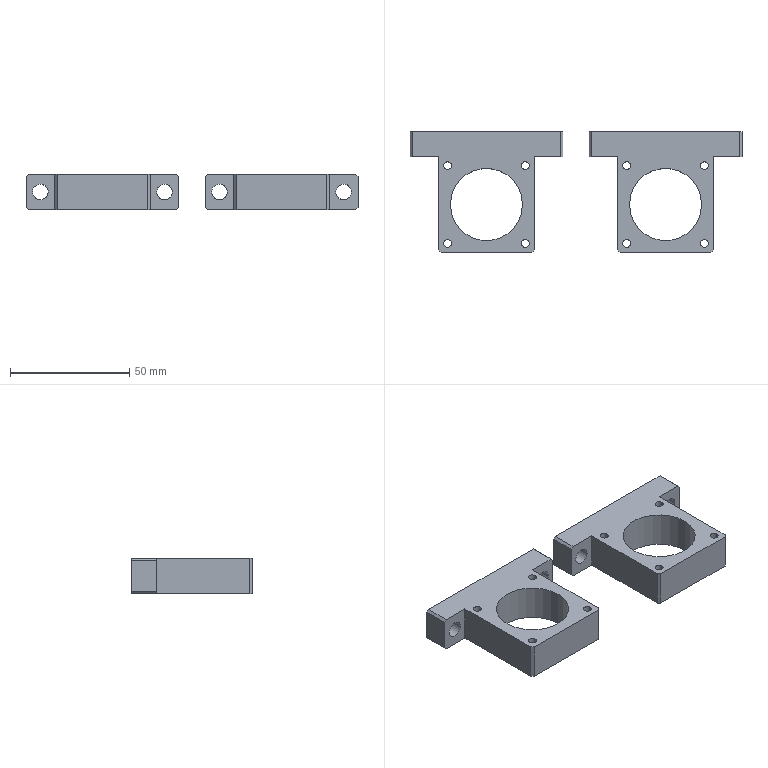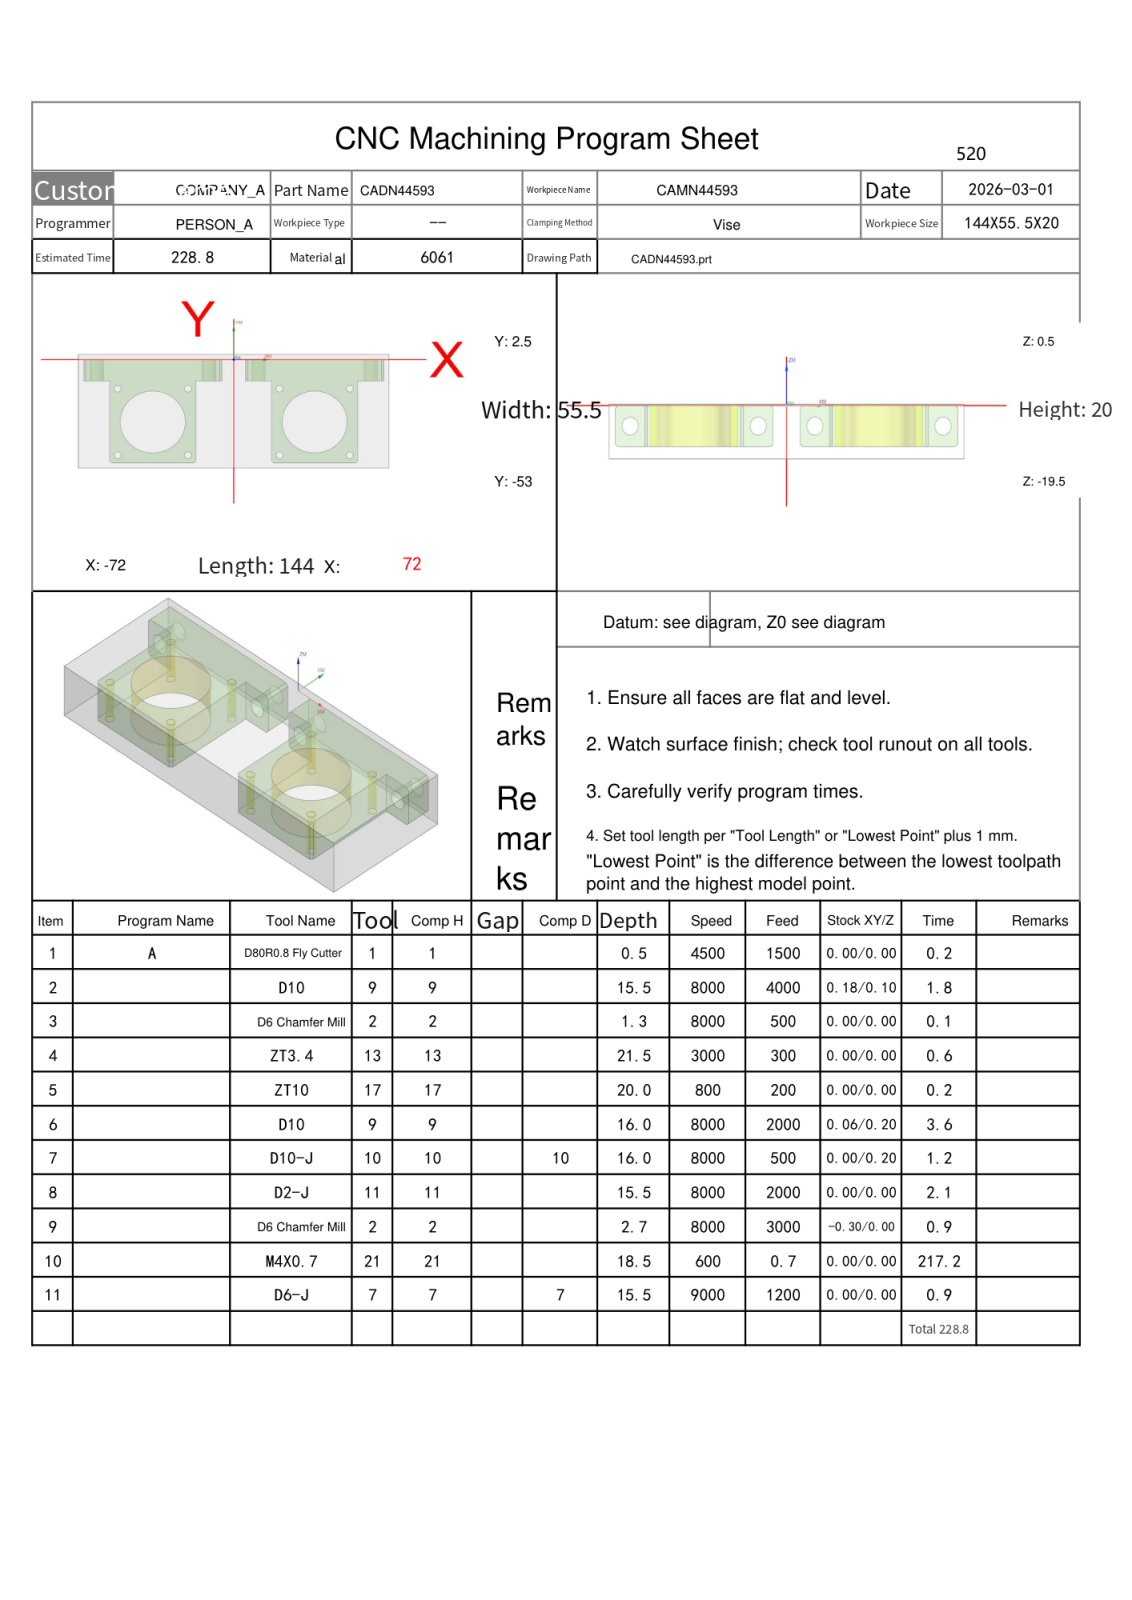NC program | NX | posted by the shop | part box 139 x 50.5 x 15 mm
Lines 2730 to 3768 of 10033:
N8 T11 M06
(D2-J  D=2. R=0. H=11 ce=0.00 di=0.00)
G00 G90 G54 X16.3 Y-15.65 M03 S8000
G43 H11 Z50.
M08
Z0.0
G01 X16.302 Y-15.649 Z-.03 F2000.
X16.31 Y-15.647 Z-.058
X16.321 Y-15.644 Z-.082
X16.335 Y-15.639 Z-.104
X16.352 Y-15.633 Z-.123
X16.37 Y-15.625 Z-.14
X16.39 Y-15.615 Z-.154
X16.41 Y-15.603 Z-.166
X16.43 Y-15.589 Z-.176
X16.448 Y-15.572 Z-.184
X16.465 Y-15.553 Z-.19
X16.479 Y-15.532 Z-.195
X16.49 Y-15.507 Z-.198
X16.497 Y-15.48 Z-.199
X16.5 Y-15.45 Z-.2
Y-11.5
X12.551
X12.536 Y-11.514 Z-.201
X12.547 Y-11.556 Z-.202
X12.581 Y-11.621 Z-.205
X12.636 Y-11.709 Z-.209
X12.901 Y-12.065 Z-.225
X13.155 Y-12.378 Z-.239
X13.354 Y-12.611 Z-.249
X13.591 Y-12.875 Z-.262
X13.868 Y-13.174 Z-.276
X14.178 Y-13.495 Z-.292
X14.505 Y-13.822 Z-.308
X14.826 Y-14.132 Z-.324
X15.125 Y-14.409 Z-.338
X15.389 Y-14.646 Z-.351
X15.622 Y-14.845 Z-.361
X15.935 Y-15.099 Z-.375
X16.291 Y-15.364 Z-.391
X16.379 Y-15.419 Z-.395
X16.444 Y-15.453 Z-.398
X16.486 Y-15.464 Z-.399
X16.5 Y-15.45 Z-.4
Y-11.5
X12.55
X12.536 Y-11.514 Z-.401
X12.547 Y-11.556 Z-.402
X12.581 Y-11.621 Z-.405
X12.636 Y-11.709 Z-.409
X12.901 Y-12.065 Z-.425
X13.155 Y-12.378 Z-.439
X13.354 Y-12.611 Z-.449
X13.591 Y-12.875 Z-.462
X13.868 Y-13.174 Z-.476
X14.178 Y-13.495 Z-.492
X14.505 Y-13.822 Z-.508
X14.826 Y-14.132 Z-.524
X15.125 Y-14.409 Z-.538
X15.389 Y-14.646 Z-.551
X15.622 Y-14.845 Z-.561
X15.935 Y-15.099 Z-.575
X16.291 Y-15.364 Z-.591
X16.379 Y-15.419 Z-.595
X16.444 Y-15.453 Z-.598
X16.486 Y-15.464 Z-.599
X16.5 Y-15.45 Z-.6
Y-11.5
X12.55
X12.536 Y-11.514 Z-.601
X12.547 Y-11.556 Z-.602
X12.581 Y-11.621 Z-.605
X12.636 Y-11.709 Z-.609
X12.901 Y-12.065 Z-.625
X13.155 Y-12.378 Z-.639
X13.354 Y-12.611 Z-.649
X13.591 Y-12.875 Z-.662
X13.868 Y-13.174 Z-.676
X14.178 Y-13.495 Z-.692
X14.505 Y-13.822 Z-.708
X14.826 Y-14.132 Z-.724
X15.125 Y-14.409 Z-.738
X15.389 Y-14.646 Z-.751
X15.622 Y-14.845 Z-.761
X15.935 Y-15.099 Z-.775
X16.291 Y-15.364 Z-.791
X16.379 Y-15.419 Z-.795
X16.444 Y-15.453 Z-.798
X16.486 Y-15.464 Z-.799
X16.5 Y-15.45 Z-.8
Y-11.5
X12.55
X12.536 Y-11.514 Z-.801
X12.547 Y-11.556 Z-.802
X12.581 Y-11.621 Z-.805
X12.636 Y-11.709 Z-.809
X12.901 Y-12.065 Z-.825
X13.155 Y-12.378 Z-.839
X13.354 Y-12.611 Z-.849
X13.591 Y-12.875 Z-.862
X13.868 Y-13.174 Z-.876
X14.178 Y-13.495 Z-.892
X14.505 Y-13.822 Z-.908
X14.826 Y-14.132 Z-.924
X15.125 Y-14.409 Z-.938
X15.389 Y-14.646 Z-.951
X15.622 Y-14.845 Z-.961
X15.935 Y-15.099 Z-.975
X16.291 Y-15.364 Z-.991
X16.379 Y-15.419 Z-.995
X16.444 Y-15.453 Z-.998
X16.486 Y-15.464 Z-.999
X16.5 Y-15.45 Z-1.
Y-11.5
X12.55
X12.536 Y-11.514 Z-1.001
X12.547 Y-11.556 Z-1.002
X12.581 Y-11.621 Z-1.005
X12.636 Y-11.709 Z-1.009
X12.901 Y-12.065 Z-1.025
X13.155 Y-12.378 Z-1.039
X13.354 Y-12.611 Z-1.049
X13.591 Y-12.875 Z-1.062
X13.868 Y-13.174 Z-1.076
X14.178 Y-13.495 Z-1.092
X14.505 Y-13.822 Z-1.108
X14.826 Y-14.132 Z-1.124
X15.125 Y-14.409 Z-1.138
X15.389 Y-14.646 Z-1.151
X15.622 Y-14.845 Z-1.161
X15.935 Y-15.099 Z-1.175
X16.291 Y-15.364 Z-1.191
X16.379 Y-15.419 Z-1.195
X16.444 Y-15.453 Z-1.198
X16.486 Y-15.464 Z-1.199
X16.5 Y-15.45 Z-1.2
Y-11.5
X12.55
X12.536 Y-11.514 Z-1.201
X12.547 Y-11.556 Z-1.202
X12.581 Y-11.621 Z-1.205
X12.636 Y-11.709 Z-1.209
X12.901 Y-12.065 Z-1.225
X13.155 Y-12.378 Z-1.239
X13.354 Y-12.611 Z-1.249
X13.591 Y-12.875 Z-1.262
X13.868 Y-13.174 Z-1.276
X14.178 Y-13.495 Z-1.292
X14.505 Y-13.822 Z-1.308
X14.826 Y-14.132 Z-1.324
X15.125 Y-14.409 Z-1.338
X15.389 Y-14.646 Z-1.351
X15.622 Y-14.845 Z-1.361
X15.935 Y-15.099 Z-1.375
X16.291 Y-15.364 Z-1.391
X16.379 Y-15.419 Z-1.395
X16.444 Y-15.453 Z-1.398
X16.486 Y-15.464 Z-1.399
X16.5 Y-15.45 Z-1.4
Y-11.5
X12.55
X12.536 Y-11.514 Z-1.401
X12.547 Y-11.556 Z-1.402
X12.581 Y-11.621 Z-1.405
X12.636 Y-11.709 Z-1.409
X12.901 Y-12.065 Z-1.425
X13.155 Y-12.378 Z-1.439
X13.354 Y-12.611 Z-1.449
X13.591 Y-12.875 Z-1.462
X13.868 Y-13.174 Z-1.476
X14.178 Y-13.495 Z-1.492
X14.505 Y-13.822 Z-1.508
X14.826 Y-14.132 Z-1.524
X15.125 Y-14.409 Z-1.538
X15.389 Y-14.646 Z-1.551
X15.622 Y-14.845 Z-1.561
X15.935 Y-15.099 Z-1.575
X16.291 Y-15.364 Z-1.591
X16.379 Y-15.419 Z-1.595
X16.444 Y-15.453 Z-1.598
X16.486 Y-15.464 Z-1.599
X16.5 Y-15.45 Z-1.6
Y-11.5
X12.55
X12.536 Y-11.514 Z-1.601
X12.547 Y-11.556 Z-1.602
X12.581 Y-11.621 Z-1.605
X12.636 Y-11.709 Z-1.609
X12.901 Y-12.065 Z-1.625
X13.155 Y-12.378 Z-1.639
X13.354 Y-12.611 Z-1.649
X13.591 Y-12.875 Z-1.662
X13.868 Y-13.174 Z-1.676
X14.178 Y-13.495 Z-1.692
X14.505 Y-13.822 Z-1.708
X14.826 Y-14.132 Z-1.724
X15.125 Y-14.409 Z-1.738
X15.389 Y-14.646 Z-1.751
X15.622 Y-14.845 Z-1.761
X15.935 Y-15.099 Z-1.775
X16.291 Y-15.364 Z-1.791
X16.379 Y-15.419 Z-1.795
X16.444 Y-15.453 Z-1.798
X16.486 Y-15.464 Z-1.799
X16.5 Y-15.45 Z-1.8
Y-11.5
X12.55
X12.536 Y-11.514 Z-1.801
X12.547 Y-11.556 Z-1.802
X12.581 Y-11.621 Z-1.805
X12.636 Y-11.709 Z-1.809
X12.901 Y-12.065 Z-1.825
X13.155 Y-12.378 Z-1.839
X13.354 Y-12.611 Z-1.849
X13.591 Y-12.875 Z-1.862
X13.868 Y-13.174 Z-1.876
X14.178 Y-13.495 Z-1.892
X14.505 Y-13.822 Z-1.908
X14.826 Y-14.132 Z-1.924
X15.125 Y-14.409 Z-1.938
X15.389 Y-14.646 Z-1.951
X15.622 Y-14.845 Z-1.961
X15.935 Y-15.099 Z-1.975
X16.291 Y-15.364 Z-1.991
X16.379 Y-15.419 Z-1.995
X16.444 Y-15.453 Z-1.998
X16.486 Y-15.464 Z-1.999
X16.5 Y-15.45 Z-2.
Y-11.5
X12.55
X12.536 Y-11.514 Z-2.001
X12.547 Y-11.556 Z-2.002
X12.581 Y-11.621 Z-2.005
X12.636 Y-11.709 Z-2.009
X12.901 Y-12.065 Z-2.025
X13.155 Y-12.378 Z-2.039
X13.354 Y-12.611 Z-2.049
X13.591 Y-12.875 Z-2.062
X13.868 Y-13.174 Z-2.076
X14.178 Y-13.495 Z-2.092
X14.505 Y-13.822 Z-2.108
X14.826 Y-14.132 Z-2.124
X15.125 Y-14.409 Z-2.138
X15.389 Y-14.646 Z-2.151
X15.622 Y-14.845 Z-2.161
X15.935 Y-15.099 Z-2.175
X16.291 Y-15.364 Z-2.191
X16.379 Y-15.419 Z-2.195
X16.444 Y-15.453 Z-2.198
X16.486 Y-15.464 Z-2.199
X16.5 Y-15.45 Z-2.2
Y-11.5
X12.55
X12.536 Y-11.514 Z-2.201
X12.547 Y-11.556 Z-2.202
X12.581 Y-11.621 Z-2.205
X12.636 Y-11.709 Z-2.209
X12.901 Y-12.065 Z-2.225
X13.155 Y-12.378 Z-2.239
X13.354 Y-12.611 Z-2.249
X13.591 Y-12.875 Z-2.262
X13.868 Y-13.174 Z-2.276
X14.178 Y-13.495 Z-2.292
X14.505 Y-13.822 Z-2.308
X14.826 Y-14.132 Z-2.324
X15.125 Y-14.409 Z-2.338
X15.389 Y-14.646 Z-2.351
X15.622 Y-14.845 Z-2.361
X15.935 Y-15.099 Z-2.375
X16.291 Y-15.364 Z-2.391
X16.379 Y-15.419 Z-2.395
X16.444 Y-15.453 Z-2.398
X16.486 Y-15.464 Z-2.399
X16.5 Y-15.45 Z-2.4
Y-11.5
X12.55
X12.536 Y-11.514 Z-2.401
X12.547 Y-11.556 Z-2.402
X12.581 Y-11.621 Z-2.405
X12.636 Y-11.709 Z-2.409
X12.901 Y-12.065 Z-2.425
X13.155 Y-12.378 Z-2.439
X13.354 Y-12.611 Z-2.449
X13.591 Y-12.875 Z-2.462
X13.868 Y-13.174 Z-2.476
X14.178 Y-13.495 Z-2.492
X14.505 Y-13.822 Z-2.508
X14.826 Y-14.132 Z-2.524
X15.125 Y-14.409 Z-2.538
X15.389 Y-14.646 Z-2.551
X15.622 Y-14.845 Z-2.561
X15.935 Y-15.099 Z-2.575
X16.291 Y-15.364 Z-2.591
X16.379 Y-15.419 Z-2.595
X16.444 Y-15.453 Z-2.598
X16.486 Y-15.464 Z-2.599
X16.5 Y-15.45 Z-2.6
Y-11.5
X12.55
X12.536 Y-11.514 Z-2.601
X12.547 Y-11.556 Z-2.602
X12.581 Y-11.621 Z-2.605
X12.636 Y-11.709 Z-2.609
X12.901 Y-12.065 Z-2.625
X13.155 Y-12.378 Z-2.639
X13.354 Y-12.611 Z-2.649
X13.591 Y-12.875 Z-2.662
X13.868 Y-13.174 Z-2.676
X14.178 Y-13.495 Z-2.692
X14.505 Y-13.822 Z-2.708
X14.826 Y-14.132 Z-2.724
X15.125 Y-14.409 Z-2.738
X15.389 Y-14.646 Z-2.751
X15.622 Y-14.845 Z-2.761
X15.935 Y-15.099 Z-2.775
X16.291 Y-15.364 Z-2.791
X16.379 Y-15.419 Z-2.795
X16.444 Y-15.453 Z-2.798
X16.486 Y-15.464 Z-2.799
X16.5 Y-15.45 Z-2.8
Y-11.5
X12.55
X12.536 Y-11.514 Z-2.801
X12.547 Y-11.556 Z-2.802
X12.581 Y-11.621 Z-2.805
X12.636 Y-11.709 Z-2.809
X12.901 Y-12.065 Z-2.825
X13.155 Y-12.378 Z-2.839
X13.354 Y-12.611 Z-2.849
X13.591 Y-12.875 Z-2.862
X13.868 Y-13.174 Z-2.876
X14.178 Y-13.495 Z-2.892
X14.505 Y-13.822 Z-2.908
X14.826 Y-14.132 Z-2.924
X15.125 Y-14.409 Z-2.938
X15.389 Y-14.646 Z-2.951
X15.622 Y-14.845 Z-2.961
X15.935 Y-15.099 Z-2.975
X16.291 Y-15.364 Z-2.991
X16.379 Y-15.419 Z-2.995
X16.444 Y-15.453 Z-2.998
X16.486 Y-15.464 Z-2.999
X16.5 Y-15.45 Z-3.
Y-11.5
X12.55
X12.536 Y-11.514 Z-3.001
X12.547 Y-11.556 Z-3.002
X12.581 Y-11.621 Z-3.005
X12.636 Y-11.709 Z-3.009
X12.901 Y-12.065 Z-3.025
X13.155 Y-12.378 Z-3.039
X13.354 Y-12.611 Z-3.049
X13.591 Y-12.875 Z-3.062
X13.868 Y-13.174 Z-3.076
X14.178 Y-13.495 Z-3.092
X14.505 Y-13.822 Z-3.108
X14.826 Y-14.132 Z-3.124
X15.125 Y-14.409 Z-3.138
X15.389 Y-14.646 Z-3.151
X15.622 Y-14.845 Z-3.161
X15.935 Y-15.099 Z-3.175
X16.291 Y-15.364 Z-3.191
X16.379 Y-15.419 Z-3.195
X16.444 Y-15.453 Z-3.198
X16.486 Y-15.464 Z-3.199
X16.5 Y-15.45 Z-3.2
Y-11.5
X12.55
X12.536 Y-11.514 Z-3.201
X12.547 Y-11.556 Z-3.202
X12.581 Y-11.621 Z-3.205
X12.636 Y-11.709 Z-3.209
X12.901 Y-12.065 Z-3.225
X13.155 Y-12.378 Z-3.239
X13.354 Y-12.611 Z-3.249
X13.591 Y-12.875 Z-3.262
X13.868 Y-13.174 Z-3.276
X14.178 Y-13.495 Z-3.292
X14.505 Y-13.822 Z-3.308
X14.826 Y-14.132 Z-3.324
X15.125 Y-14.409 Z-3.338
X15.389 Y-14.646 Z-3.351
X15.622 Y-14.845 Z-3.361
X15.935 Y-15.099 Z-3.375
X16.291 Y-15.364 Z-3.391
X16.379 Y-15.419 Z-3.395
X16.444 Y-15.453 Z-3.398
X16.486 Y-15.464 Z-3.399
X16.5 Y-15.45 Z-3.4
Y-11.5
X12.55
X12.536 Y-11.514 Z-3.401
X12.547 Y-11.556 Z-3.402
X12.581 Y-11.621 Z-3.405
X12.636 Y-11.709 Z-3.409
X12.901 Y-12.065 Z-3.425
X13.155 Y-12.378 Z-3.439
X13.354 Y-12.611 Z-3.449
X13.591 Y-12.875 Z-3.462
X13.868 Y-13.174 Z-3.476
X14.178 Y-13.495 Z-3.492
X14.505 Y-13.822 Z-3.508
X14.826 Y-14.132 Z-3.524
X15.125 Y-14.409 Z-3.538
X15.389 Y-14.646 Z-3.551
X15.622 Y-14.845 Z-3.561
X15.935 Y-15.099 Z-3.575
X16.291 Y-15.364 Z-3.591
X16.379 Y-15.419 Z-3.595
X16.444 Y-15.453 Z-3.598
X16.486 Y-15.464 Z-3.599
X16.5 Y-15.45 Z-3.6
Y-11.5
X12.55
X12.536 Y-11.514 Z-3.601
X12.547 Y-11.556 Z-3.602
X12.581 Y-11.621 Z-3.605
X12.636 Y-11.709 Z-3.609
X12.901 Y-12.065 Z-3.625
X13.155 Y-12.378 Z-3.639
X13.354 Y-12.611 Z-3.649
X13.591 Y-12.875 Z-3.662
X13.868 Y-13.174 Z-3.676
X14.178 Y-13.495 Z-3.692
X14.505 Y-13.822 Z-3.708
X14.826 Y-14.132 Z-3.724
X15.125 Y-14.409 Z-3.738
X15.389 Y-14.646 Z-3.751
X15.622 Y-14.845 Z-3.761
X15.935 Y-15.099 Z-3.775
X16.291 Y-15.364 Z-3.791
X16.379 Y-15.419 Z-3.795
X16.444 Y-15.453 Z-3.798
X16.486 Y-15.464 Z-3.799
X16.5 Y-15.45 Z-3.8
Y-11.5
X12.55
X12.536 Y-11.514 Z-3.801
X12.547 Y-11.556 Z-3.802
X12.581 Y-11.621 Z-3.805
X12.636 Y-11.709 Z-3.809
X12.901 Y-12.065 Z-3.825
X13.155 Y-12.378 Z-3.839
X13.354 Y-12.611 Z-3.849
X13.591 Y-12.875 Z-3.862
X13.868 Y-13.174 Z-3.876
X14.178 Y-13.495 Z-3.892
X14.505 Y-13.822 Z-3.908
X14.826 Y-14.132 Z-3.924
X15.125 Y-14.409 Z-3.938
X15.389 Y-14.646 Z-3.951
X15.622 Y-14.845 Z-3.961
X15.935 Y-15.099 Z-3.975
X16.291 Y-15.364 Z-3.991
X16.379 Y-15.419 Z-3.995
X16.444 Y-15.453 Z-3.998
X16.486 Y-15.464 Z-3.999
X16.5 Y-15.45 Z-4.
Y-11.5
X12.55
X12.536 Y-11.514 Z-4.001
X12.547 Y-11.556 Z-4.002
X12.581 Y-11.621 Z-4.005
X12.636 Y-11.709 Z-4.009
X12.901 Y-12.065 Z-4.025
X13.155 Y-12.378 Z-4.039
X13.354 Y-12.611 Z-4.049
X13.591 Y-12.875 Z-4.062
X13.868 Y-13.174 Z-4.076
X14.178 Y-13.495 Z-4.092
X14.505 Y-13.822 Z-4.108
X14.826 Y-14.132 Z-4.124
X15.125 Y-14.409 Z-4.138
X15.389 Y-14.646 Z-4.151
X15.622 Y-14.845 Z-4.161
X15.935 Y-15.099 Z-4.175
X16.291 Y-15.364 Z-4.191
X16.379 Y-15.419 Z-4.195
X16.444 Y-15.453 Z-4.198
X16.486 Y-15.464 Z-4.199
X16.5 Y-15.45 Z-4.2
Y-11.5
X12.55
X12.536 Y-11.514 Z-4.201
X12.547 Y-11.556 Z-4.202
X12.581 Y-11.621 Z-4.205
X12.636 Y-11.709 Z-4.209
X12.901 Y-12.065 Z-4.225
X13.155 Y-12.378 Z-4.239
X13.354 Y-12.611 Z-4.249
X13.591 Y-12.875 Z-4.262
X13.868 Y-13.174 Z-4.276
X14.178 Y-13.495 Z-4.292
X14.505 Y-13.822 Z-4.308
X14.826 Y-14.132 Z-4.324
X15.125 Y-14.409 Z-4.338
X15.389 Y-14.646 Z-4.351
X15.622 Y-14.845 Z-4.361
X15.935 Y-15.099 Z-4.375
X16.291 Y-15.364 Z-4.391
X16.379 Y-15.419 Z-4.395
X16.444 Y-15.453 Z-4.398
X16.486 Y-15.464 Z-4.399
X16.5 Y-15.45 Z-4.4
Y-11.5
X12.55
X12.536 Y-11.514 Z-4.401
X12.547 Y-11.556 Z-4.402
X12.581 Y-11.621 Z-4.405
X12.636 Y-11.709 Z-4.409
X12.901 Y-12.065 Z-4.425
X13.155 Y-12.378 Z-4.439
X13.354 Y-12.611 Z-4.449
X13.591 Y-12.875 Z-4.462
X13.868 Y-13.174 Z-4.476
X14.178 Y-13.495 Z-4.492
X14.505 Y-13.822 Z-4.508
X14.826 Y-14.132 Z-4.524
X15.125 Y-14.409 Z-4.538
X15.389 Y-14.646 Z-4.551
X15.622 Y-14.845 Z-4.561
X15.935 Y-15.099 Z-4.575
X16.291 Y-15.364 Z-4.591
X16.379 Y-15.419 Z-4.595
X16.444 Y-15.453 Z-4.598
X16.486 Y-15.464 Z-4.599
X16.5 Y-15.45 Z-4.6
Y-11.5
X12.55
X12.536 Y-11.514 Z-4.601
X12.547 Y-11.556 Z-4.602
X12.581 Y-11.621 Z-4.605
X12.636 Y-11.709 Z-4.609
X12.901 Y-12.065 Z-4.625
X13.155 Y-12.378 Z-4.639
X13.354 Y-12.611 Z-4.649
X13.591 Y-12.875 Z-4.662
X13.868 Y-13.174 Z-4.676
X14.178 Y-13.495 Z-4.692
X14.505 Y-13.822 Z-4.708
X14.826 Y-14.132 Z-4.724
X15.125 Y-14.409 Z-4.738
X15.389 Y-14.646 Z-4.751
X15.622 Y-14.845 Z-4.761
X15.935 Y-15.099 Z-4.775
X16.291 Y-15.364 Z-4.791
X16.379 Y-15.419 Z-4.795
X16.444 Y-15.453 Z-4.798
X16.486 Y-15.464 Z-4.799
X16.5 Y-15.45 Z-4.8
Y-11.5
X12.55
X12.536 Y-11.514 Z-4.801
X12.547 Y-11.556 Z-4.802
X12.581 Y-11.621 Z-4.805
X12.636 Y-11.709 Z-4.809
X12.901 Y-12.065 Z-4.825
X13.155 Y-12.378 Z-4.839
X13.354 Y-12.611 Z-4.849
X13.591 Y-12.875 Z-4.862
X13.868 Y-13.174 Z-4.876
X14.178 Y-13.495 Z-4.892
X14.505 Y-13.822 Z-4.908
X14.826 Y-14.132 Z-4.924
X15.125 Y-14.409 Z-4.938
X15.389 Y-14.646 Z-4.951
X15.622 Y-14.845 Z-4.961
X15.935 Y-15.099 Z-4.975
X16.291 Y-15.364 Z-4.991
X16.379 Y-15.419 Z-4.995
X16.444 Y-15.453 Z-4.998
X16.486 Y-15.464 Z-4.999
X16.5 Y-15.45 Z-5.
Y-11.5
X12.55
X12.536 Y-11.514 Z-5.001
X12.547 Y-11.556 Z-5.002
X12.581 Y-11.621 Z-5.005
X12.636 Y-11.709 Z-5.009
X12.901 Y-12.065 Z-5.025
X13.155 Y-12.378 Z-5.039
X13.354 Y-12.611 Z-5.049
X13.591 Y-12.875 Z-5.062
X13.868 Y-13.174 Z-5.076
X14.178 Y-13.495 Z-5.092
X14.505 Y-13.822 Z-5.108
X14.826 Y-14.132 Z-5.124
X15.125 Y-14.409 Z-5.138
X15.389 Y-14.646 Z-5.151
X15.622 Y-14.845 Z-5.161
X15.935 Y-15.099 Z-5.175
X16.291 Y-15.364 Z-5.191
X16.379 Y-15.419 Z-5.195
X16.444 Y-15.453 Z-5.198
X16.486 Y-15.464 Z-5.199
X16.5 Y-15.45 Z-5.2
Y-11.5
X12.55
X12.536 Y-11.514 Z-5.201
X12.547 Y-11.556 Z-5.202
X12.581 Y-11.621 Z-5.205
X12.636 Y-11.709 Z-5.209
X12.901 Y-12.065 Z-5.225
X13.155 Y-12.378 Z-5.239
X13.354 Y-12.611 Z-5.249
X13.591 Y-12.875 Z-5.262
X13.868 Y-13.174 Z-5.276
X14.178 Y-13.495 Z-5.292
X14.505 Y-13.822 Z-5.308
X14.826 Y-14.132 Z-5.324
X15.125 Y-14.409 Z-5.338
X15.389 Y-14.646 Z-5.351
X15.622 Y-14.845 Z-5.361
X15.935 Y-15.099 Z-5.375
X16.291 Y-15.364 Z-5.391
X16.379 Y-15.419 Z-5.395
X16.444 Y-15.453 Z-5.398
X16.486 Y-15.464 Z-5.399
X16.5 Y-15.45 Z-5.4
Y-11.5
X12.55
X12.536 Y-11.514 Z-5.401
X12.547 Y-11.556 Z-5.402
X12.581 Y-11.621 Z-5.405
X12.636 Y-11.709 Z-5.409
X12.901 Y-12.065 Z-5.425
X13.155 Y-12.378 Z-5.439
X13.354 Y-12.611 Z-5.449
X13.591 Y-12.875 Z-5.462
X13.868 Y-13.174 Z-5.476
X14.178 Y-13.495 Z-5.492
X14.505 Y-13.822 Z-5.508
X14.826 Y-14.132 Z-5.524
X15.125 Y-14.409 Z-5.538
X15.389 Y-14.646 Z-5.551
X15.622 Y-14.845 Z-5.561
X15.935 Y-15.099 Z-5.575
X16.291 Y-15.364 Z-5.591
X16.379 Y-15.419 Z-5.595
X16.444 Y-15.453 Z-5.598
X16.486 Y-15.464 Z-5.599
X16.5 Y-15.45 Z-5.6
Y-11.5
X12.55
X12.536 Y-11.514 Z-5.601
X12.547 Y-11.556 Z-5.602
X12.581 Y-11.621 Z-5.605
X12.636 Y-11.709 Z-5.609
X12.901 Y-12.065 Z-5.625
X13.155 Y-12.378 Z-5.639
X13.354 Y-12.611 Z-5.649
X13.591 Y-12.875 Z-5.662
X13.868 Y-13.174 Z-5.676
X14.178 Y-13.495 Z-5.692
X14.505 Y-13.822 Z-5.708
X14.826 Y-14.132 Z-5.724
X15.125 Y-14.409 Z-5.738
X15.389 Y-14.646 Z-5.751
X15.622 Y-14.845 Z-5.761
X15.935 Y-15.099 Z-5.775
X16.291 Y-15.364 Z-5.791
X16.379 Y-15.419 Z-5.795
X16.444 Y-15.453 Z-5.798
X16.486 Y-15.464 Z-5.799
X16.5 Y-15.45 Z-5.8
Y-11.5
X12.55
X12.536 Y-11.514 Z-5.801
X12.547 Y-11.556 Z-5.802
X12.581 Y-11.621 Z-5.805
X12.636 Y-11.709 Z-5.809
X12.901 Y-12.065 Z-5.825
X13.155 Y-12.378 Z-5.839
X13.354 Y-12.611 Z-5.849
X13.591 Y-12.875 Z-5.862
X13.868 Y-13.174 Z-5.876
X14.178 Y-13.495 Z-5.892
X14.505 Y-13.822 Z-5.908
X14.826 Y-14.132 Z-5.924
X15.125 Y-14.409 Z-5.938
X15.389 Y-14.646 Z-5.951
X15.622 Y-14.845 Z-5.961
X15.935 Y-15.099 Z-5.975
X16.291 Y-15.364 Z-5.991
X16.379 Y-15.419 Z-5.995
X16.444 Y-15.453 Z-5.998
X16.486 Y-15.464 Z-5.999
X16.5 Y-15.45 Z-6.
Y-11.5
X12.55
X12.536 Y-11.514 Z-6.001
X12.547 Y-11.556 Z-6.002
X12.581 Y-11.621 Z-6.005
X12.636 Y-11.709 Z-6.009
X12.901 Y-12.065 Z-6.025
X13.155 Y-12.378 Z-6.039
X13.354 Y-12.611 Z-6.049
X13.591 Y-12.875 Z-6.062
X13.868 Y-13.174 Z-6.076
X14.178 Y-13.495 Z-6.092
X14.505 Y-13.822 Z-6.108
X14.826 Y-14.132 Z-6.124
X15.125 Y-14.409 Z-6.138
X15.389 Y-14.646 Z-6.151
X15.622 Y-14.845 Z-6.161
X15.935 Y-15.099 Z-6.175
X16.291 Y-15.364 Z-6.191
X16.379 Y-15.419 Z-6.195
X16.444 Y-15.453 Z-6.198
X16.486 Y-15.464 Z-6.199
X16.5 Y-15.45 Z-6.2
Y-11.5
X12.55
X12.536 Y-11.514 Z-6.201
X12.547 Y-11.556 Z-6.202
X12.581 Y-11.621 Z-6.205
X12.636 Y-11.709 Z-6.209
X12.901 Y-12.065 Z-6.225
X13.155 Y-12.378 Z-6.239
X13.354 Y-12.611 Z-6.249
X13.591 Y-12.875 Z-6.262
X13.868 Y-13.174 Z-6.276
X14.178 Y-13.495 Z-6.292
X14.505 Y-13.822 Z-6.308
X14.826 Y-14.132 Z-6.324
X15.125 Y-14.409 Z-6.338
X15.389 Y-14.646 Z-6.351
X15.622 Y-14.845 Z-6.361
X15.935 Y-15.099 Z-6.375
X16.291 Y-15.364 Z-6.391
X16.379 Y-15.419 Z-6.395
X16.444 Y-15.453 Z-6.398
X16.486 Y-15.464 Z-6.399
X16.5 Y-15.45 Z-6.4
Y-11.5
X12.55
X12.536 Y-11.514 Z-6.401
X12.547 Y-11.556 Z-6.402
X12.581 Y-11.621 Z-6.405
X12.636 Y-11.709 Z-6.409
X12.901 Y-12.065 Z-6.425
X13.155 Y-12.378 Z-6.439
X13.354 Y-12.611 Z-6.449
X13.591 Y-12.875 Z-6.462
X13.868 Y-13.174 Z-6.476
X14.178 Y-13.495 Z-6.492
X14.505 Y-13.822 Z-6.508
X14.826 Y-14.132 Z-6.524
X15.125 Y-14.409 Z-6.538
X15.389 Y-14.646 Z-6.551
X15.622 Y-14.845 Z-6.561
X15.935 Y-15.099 Z-6.575
X16.291 Y-15.364 Z-6.591
X16.379 Y-15.419 Z-6.595
X16.444 Y-15.453 Z-6.598
X16.486 Y-15.464 Z-6.599
X16.5 Y-15.45 Z-6.6
Y-11.5
X12.55
X12.536 Y-11.514 Z-6.601
X12.547 Y-11.556 Z-6.602
X12.581 Y-11.621 Z-6.605
X12.636 Y-11.709 Z-6.609
X12.901 Y-12.065 Z-6.625
X13.155 Y-12.378 Z-6.639
X13.354 Y-12.611 Z-6.649
X13.591 Y-12.875 Z-6.662
X13.868 Y-13.174 Z-6.676
X14.178 Y-13.495 Z-6.692
X14.505 Y-13.822 Z-6.708
X14.826 Y-14.132 Z-6.724
X15.125 Y-14.409 Z-6.738
X15.389 Y-14.646 Z-6.751
X15.622 Y-14.845 Z-6.761
X15.935 Y-15.099 Z-6.775
X16.291 Y-15.364 Z-6.791
X16.379 Y-15.419 Z-6.795
X16.444 Y-15.453 Z-6.798
X16.486 Y-15.464 Z-6.799
X16.5 Y-15.45 Z-6.8
Y-11.5
X12.55
X12.536 Y-11.514 Z-6.801
X12.547 Y-11.556 Z-6.802
X12.581 Y-11.621 Z-6.805
X12.636 Y-11.709 Z-6.809
X12.901 Y-12.065 Z-6.825
X13.155 Y-12.378 Z-6.839
X13.354 Y-12.611 Z-6.849
X13.591 Y-12.875 Z-6.862
X13.868 Y-13.174 Z-6.876
X14.178 Y-13.495 Z-6.892
X14.505 Y-13.822 Z-6.908
X14.826 Y-14.132 Z-6.924
X15.125 Y-14.409 Z-6.938
X15.389 Y-14.646 Z-6.951
X15.622 Y-14.845 Z-6.961
X15.935 Y-15.099 Z-6.975
X16.291 Y-15.364 Z-6.991
X16.379 Y-15.419 Z-6.995
X16.444 Y-15.453 Z-6.998
X16.486 Y-15.464 Z-6.999
X16.5 Y-15.45 Z-7.
Y-11.5
X12.55
X12.536 Y-11.514 Z-7.001
X12.547 Y-11.556 Z-7.002
X12.581 Y-11.621 Z-7.005
X12.636 Y-11.709 Z-7.009
X12.901 Y-12.065 Z-7.025
X13.155 Y-12.378 Z-7.039
X13.354 Y-12.611 Z-7.049
X13.591 Y-12.875 Z-7.062
X13.868 Y-13.174 Z-7.076
X14.178 Y-13.495 Z-7.092
X14.505 Y-13.822 Z-7.108
X14.826 Y-14.132 Z-7.124
X15.125 Y-14.409 Z-7.138
X15.389 Y-14.646 Z-7.151
X15.622 Y-14.845 Z-7.161
X15.935 Y-15.099 Z-7.175
X16.291 Y-15.364 Z-7.191
X16.379 Y-15.419 Z-7.195
X16.444 Y-15.453 Z-7.198
X16.486 Y-15.464 Z-7.199
X16.5 Y-15.45 Z-7.2
Y-11.5
X12.55
X12.536 Y-11.514 Z-7.201
X12.547 Y-11.556 Z-7.202
X12.581 Y-11.621 Z-7.205
X12.636 Y-11.709 Z-7.209
X12.901 Y-12.065 Z-7.225
X13.155 Y-12.378 Z-7.239
X13.354 Y-12.611 Z-7.249
X13.591 Y-12.875 Z-7.262
X13.868 Y-13.174 Z-7.276
X14.178 Y-13.495 Z-7.292
X14.505 Y-13.822 Z-7.308
X14.826 Y-14.132 Z-7.324
X15.125 Y-14.409 Z-7.338
X15.389 Y-14.646 Z-7.351
X15.622 Y-14.845 Z-7.361
X15.935 Y-15.099 Z-7.375
X16.291 Y-15.364 Z-7.391
X16.379 Y-15.419 Z-7.395
X16.444 Y-15.453 Z-7.398
X16.486 Y-15.464 Z-7.399
X16.5 Y-15.45 Z-7.4
Y-11.5
X12.55
X12.536 Y-11.514 Z-7.401
X12.547 Y-11.556 Z-7.402
X12.581 Y-11.621 Z-7.405
X12.636 Y-11.709 Z-7.409
X12.901 Y-12.065 Z-7.425
X13.155 Y-12.378 Z-7.439
X13.354 Y-12.611 Z-7.449
X13.591 Y-12.875 Z-7.462
X13.868 Y-13.174 Z-7.476
X14.178 Y-13.495 Z-7.492
X14.505 Y-13.822 Z-7.508
X14.826 Y-14.132 Z-7.524
X15.125 Y-14.409 Z-7.538
X15.389 Y-14.646 Z-7.551
X15.622 Y-14.845 Z-7.561
X15.935 Y-15.099 Z-7.575
X16.291 Y-15.364 Z-7.591
X16.379 Y-15.419 Z-7.595
X16.444 Y-15.453 Z-7.598
X16.486 Y-15.464 Z-7.599
X16.5 Y-15.45 Z-7.6
Y-11.5
X12.55
X12.536 Y-11.514 Z-7.601
X12.547 Y-11.556 Z-7.602
X12.581 Y-11.621 Z-7.605
X12.636 Y-11.709 Z-7.609
X12.901 Y-12.065 Z-7.625
X13.155 Y-12.378 Z-7.639
X13.354 Y-12.611 Z-7.649
X13.591 Y-12.875 Z-7.662
X13.868 Y-13.174 Z-7.676
X14.178 Y-13.495 Z-7.692
X14.505 Y-13.822 Z-7.708
X14.826 Y-14.132 Z-7.724
X15.125 Y-14.409 Z-7.738
X15.389 Y-14.646 Z-7.751
X15.622 Y-14.845 Z-7.761
X15.935 Y-15.099 Z-7.775
X16.291 Y-15.364 Z-7.791
X16.379 Y-15.419 Z-7.795
X16.444 Y-15.453 Z-7.798
X16.486 Y-15.464 Z-7.799
X16.5 Y-15.45 Z-7.8
Y-11.5
X12.55
X12.536 Y-11.514 Z-7.801
X12.547 Y-11.556 Z-7.802
X12.581 Y-11.621 Z-7.805
X12.636 Y-11.709 Z-7.809
X12.901 Y-12.065 Z-7.825
X13.155 Y-12.378 Z-7.839
X13.354 Y-12.611 Z-7.849
X13.591 Y-12.875 Z-7.862
X13.868 Y-13.174 Z-7.876
X14.178 Y-13.495 Z-7.892
X14.505 Y-13.822 Z-7.908
X14.826 Y-14.132 Z-7.924
X15.125 Y-14.409 Z-7.938
X15.389 Y-14.646 Z-7.951
X15.622 Y-14.845 Z-7.961
X15.935 Y-15.099 Z-7.975
X16.291 Y-15.364 Z-7.991
X16.379 Y-15.419 Z-7.995
X16.444 Y-15.453 Z-7.998
X16.486 Y-15.464 Z-7.999
X16.5 Y-15.45 Z-8.
Y-11.5
X12.55
X12.536 Y-11.514 Z-8.001
X12.547 Y-11.556 Z-8.002
X12.581 Y-11.621 Z-8.005
X12.636 Y-11.709 Z-8.009
X12.901 Y-12.065 Z-8.025
X13.155 Y-12.378 Z-8.039
X13.354 Y-12.611 Z-8.049
X13.591 Y-12.875 Z-8.062
X13.868 Y-13.174 Z-8.076
X14.178 Y-13.495 Z-8.092
X14.505 Y-13.822 Z-8.108
X14.826 Y-14.132 Z-8.124
X15.125 Y-14.409 Z-8.138
X15.389 Y-14.646 Z-8.151
X15.622 Y-14.845 Z-8.161
X15.935 Y-15.099 Z-8.175
X16.291 Y-15.364 Z-8.191
X16.379 Y-15.419 Z-8.195
X16.444 Y-15.453 Z-8.198
X16.486 Y-15.464 Z-8.199
X16.5 Y-15.45 Z-8.2
Y-11.5
X12.55
X12.536 Y-11.514 Z-8.201
X12.547 Y-11.556 Z-8.202
X12.581 Y-11.621 Z-8.205
X12.636 Y-11.709 Z-8.209
X12.901 Y-12.065 Z-8.225
X13.155 Y-12.378 Z-8.239
X13.354 Y-12.611 Z-8.249
X13.591 Y-12.875 Z-8.262
X13.868 Y-13.174 Z-8.276
X14.178 Y-13.495 Z-8.292
X14.505 Y-13.822 Z-8.308
X14.826 Y-14.132 Z-8.324
X15.125 Y-14.409 Z-8.338
X15.389 Y-14.646 Z-8.351
X15.622 Y-14.845 Z-8.361
X15.935 Y-15.099 Z-8.375
X16.291 Y-15.364 Z-8.391
X16.379 Y-15.419 Z-8.395
X16.444 Y-15.453 Z-8.398
X16.486 Y-15.464 Z-8.399
X16.5 Y-15.45 Z-8.4
Y-11.5
X12.55
X12.536 Y-11.514 Z-8.401
X12.547 Y-11.556 Z-8.402
X12.581 Y-11.621 Z-8.405
X12.636 Y-11.709 Z-8.409
X12.901 Y-12.065 Z-8.425
X13.155 Y-12.378 Z-8.439
X13.354 Y-12.611 Z-8.449
X13.591 Y-12.875 Z-8.462
X13.868 Y-13.174 Z-8.476
X14.178 Y-13.495 Z-8.492
X14.505 Y-13.822 Z-8.508
X14.826 Y-14.132 Z-8.524
X15.125 Y-14.409 Z-8.538
X15.389 Y-14.646 Z-8.551
X15.622 Y-14.845 Z-8.561
X15.935 Y-15.099 Z-8.575
X16.291 Y-15.364 Z-8.591
X16.379 Y-15.419 Z-8.595
X16.444 Y-15.453 Z-8.598
X16.486 Y-15.464 Z-8.599
X16.5 Y-15.45 Z-8.6
Y-11.5
X12.55
X12.536 Y-11.514 Z-8.601
X12.547 Y-11.556 Z-8.602
X12.581 Y-11.621 Z-8.605
X12.636 Y-11.709 Z-8.609
X12.901 Y-12.065 Z-8.625
X13.155 Y-12.378 Z-8.639
X13.354 Y-12.611 Z-8.649
X13.591 Y-12.875 Z-8.662
X13.868 Y-13.174 Z-8.676
X14.178 Y-13.495 Z-8.692
X14.505 Y-13.822 Z-8.708
X14.826 Y-14.132 Z-8.724
X15.125 Y-14.409 Z-8.738
X15.389 Y-14.646 Z-8.751
X15.622 Y-14.845 Z-8.761
X15.935 Y-15.099 Z-8.775
X16.291 Y-15.364 Z-8.791
X16.379 Y-15.419 Z-8.795
X16.444 Y-15.453 Z-8.798
X16.486 Y-15.464 Z-8.799
X16.5 Y-15.45 Z-8.8
Y-11.5
X12.55
X12.536 Y-11.514 Z-8.801
X12.547 Y-11.556 Z-8.802
X12.581 Y-11.621 Z-8.805
X12.636 Y-11.709 Z-8.809
X12.901 Y-12.065 Z-8.825
X13.155 Y-12.378 Z-8.839
X13.354 Y-12.611 Z-8.849
X13.591 Y-12.875 Z-8.862
X13.868 Y-13.174 Z-8.876
X14.178 Y-13.495 Z-8.892
X14.505 Y-13.822 Z-8.908
X14.826 Y-14.132 Z-8.924
X15.125 Y-14.409 Z-8.938
X15.389 Y-14.646 Z-8.951
X15.622 Y-14.845 Z-8.961
X15.935 Y-15.099 Z-8.975
X16.291 Y-15.364 Z-8.991
X16.379 Y-15.419 Z-8.995
X16.444 Y-15.453 Z-8.998
X16.486 Y-15.464 Z-8.999
X16.5 Y-15.45 Z-9.
Y-11.5
X12.55
X12.536 Y-11.514 Z-9.001
X12.547 Y-11.556 Z-9.002
X12.581 Y-11.621 Z-9.005
X12.636 Y-11.709 Z-9.009